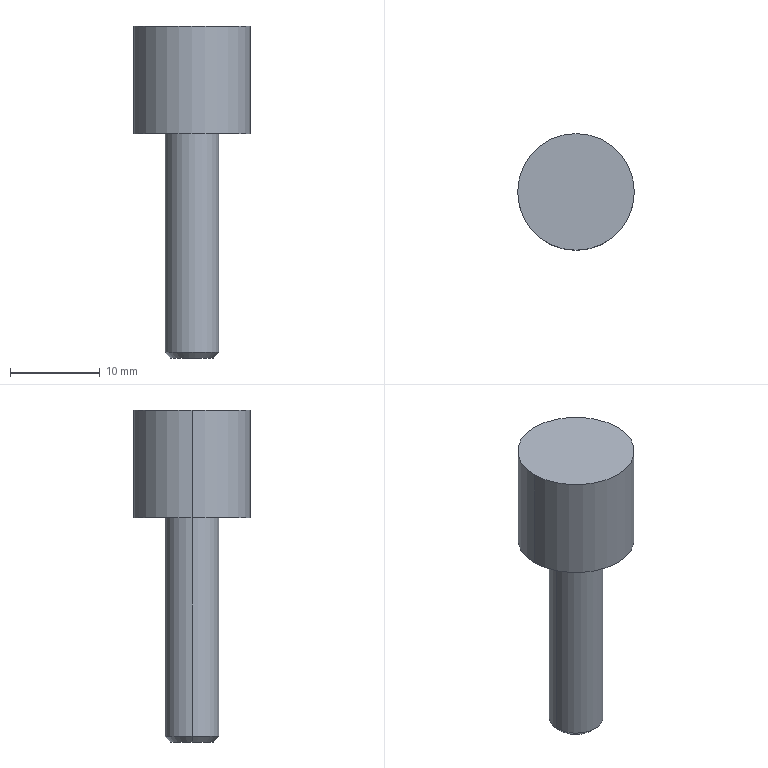Part | STEP file | LE-MX-A-TJG_PN_0007 | 1 solid | 9 faces | box 13 x 13 x 37 mm | volume 2296 mm3 | cylinder 4 | plane 3 | cone 2 | commonest cylinder face diameters 6 x2 13 x2
STEP:
#1=CARTESIAN_POINT('',(6.5,0.,0.));
#2=VERTEX_POINT('',#1);
#3=CARTESIAN_POINT('',(-6.5,0.,0.));
#4=VERTEX_POINT('',#3);
#5=CARTESIAN_POINT('',(0.,0.,0.));
#6=DIRECTION('',(0.,0.,1.));
#7=DIRECTION('',(1.,0.,0.));
#8=AXIS2_PLACEMENT_3D('',#5,#6,#7);
#9=CIRCLE('',#8,6.5);
#10=EDGE_CURVE('',#2,#4,#9,.T.);
#11=ORIENTED_EDGE('',*,*,#10,.T.);
#12=CARTESIAN_POINT('',(-6.5,0.,12.));
#13=VERTEX_POINT('',#12);
#14=CARTESIAN_POINT('',(-6.5,0.,-25.));
#15=DIRECTION('',(0.,0.,1.));
#16=VECTOR('',#15,1000.);
#17=LINE('',#14,#16);
#18=EDGE_CURVE('',#4,#13,#17,.T.);
#19=ORIENTED_EDGE('',*,*,#18,.T.);
#20=CARTESIAN_POINT('',(6.5,0.,12.));
#21=VERTEX_POINT('',#20);
#22=CARTESIAN_POINT('',(0.,0.,12.));
#23=DIRECTION('',(0.,0.,-1.));
#24=DIRECTION('',(1.,0.,0.));
#25=AXIS2_PLACEMENT_3D('',#22,#23,#24);
#26=CIRCLE('',#25,6.5);
#27=EDGE_CURVE('',#13,#21,#26,.T.);
#28=ORIENTED_EDGE('',*,*,#27,.T.);
#29=CARTESIAN_POINT('',(6.5,0.,-25.));
#30=DIRECTION('',(0.,0.,1.));
#31=VECTOR('',#30,1000.);
#32=LINE('',#29,#31);
#33=EDGE_CURVE('',#2,#21,#32,.T.);
#34=ORIENTED_EDGE('',*,*,#33,.F.);
#35=EDGE_LOOP('',(#11,#19,#28,#34));
#36=FACE_OUTER_BOUND('',#35,.T.);
#37=CARTESIAN_POINT('',(0.,0.,-25.));
#38=DIRECTION('',(0.,0.,1.));
#39=DIRECTION('',(1.,0.,0.));
#40=AXIS2_PLACEMENT_3D('',#37,#38,#39);
#41=CYLINDRICAL_SURFACE('',#40,6.5);
#42=ADVANCED_FACE('',(#36),#41,.T.);
#43=CARTESIAN_POINT('',(3.,0.,-24.387));
#44=VERTEX_POINT('',#43);
#45=CARTESIAN_POINT('',(-3.,0.,-24.387));
#46=VERTEX_POINT('',#45);
#47=CARTESIAN_POINT('',(0.,0.,-24.387));
#48=DIRECTION('',(0.,0.,1.));
#49=DIRECTION('',(1.,0.,0.));
#50=AXIS2_PLACEMENT_3D('',#47,#48,#49);
#51=CIRCLE('',#50,3.);
#52=EDGE_CURVE('',#44,#46,#51,.T.);
#53=ORIENTED_EDGE('',*,*,#52,.T.);
#54=CARTESIAN_POINT('',(-3.,0.,0.));
#55=VERTEX_POINT('',#54);
#56=CARTESIAN_POINT('',(-3.,0.,-25.));
#57=DIRECTION('',(0.,0.,1.));
#58=VECTOR('',#57,1000.);
#59=LINE('',#56,#58);
#60=EDGE_CURVE('',#46,#55,#59,.T.);
#61=ORIENTED_EDGE('',*,*,#60,.T.);
#62=CARTESIAN_POINT('',(3.,0.,0.));
#63=VERTEX_POINT('',#62);
#64=CARTESIAN_POINT('',(0.,0.,0.));
#65=DIRECTION('',(0.,0.,1.));
#66=DIRECTION('',(1.,0.,0.));
#67=AXIS2_PLACEMENT_3D('',#64,#65,#66);
#68=CIRCLE('',#67,3.);
#69=EDGE_CURVE('',#63,#55,#68,.T.);
#70=ORIENTED_EDGE('',*,*,#69,.F.);
#71=CARTESIAN_POINT('',(3.,0.,-25.));
#72=DIRECTION('',(0.,0.,1.));
#73=VECTOR('',#72,1000.);
#74=LINE('',#71,#73);
#75=EDGE_CURVE('',#44,#63,#74,.T.);
#76=ORIENTED_EDGE('',*,*,#75,.F.);
#77=EDGE_LOOP('',(#53,#61,#70,#76));
#78=FACE_OUTER_BOUND('',#77,.T.);
#79=CARTESIAN_POINT('',(0.,0.,-25.));
#80=DIRECTION('',(0.,0.,1.));
#81=DIRECTION('',(1.,0.,0.));
#82=AXIS2_PLACEMENT_3D('',#79,#80,#81);
#83=CYLINDRICAL_SURFACE('',#82,3.);
#84=ADVANCED_FACE('',(#78),#83,.T.);
#85=CARTESIAN_POINT('',(2.387,0.,-25.));
#86=VERTEX_POINT('',#85);
#87=CARTESIAN_POINT('',(-2.387,0.,-25.));
#88=VERTEX_POINT('',#87);
#89=CARTESIAN_POINT('',(0.,0.,-25.));
#90=DIRECTION('',(0.,0.,1.));
#91=DIRECTION('',(1.,0.,0.));
#92=AXIS2_PLACEMENT_3D('',#89,#90,#91);
#93=CIRCLE('',#92,2.387);
#94=EDGE_CURVE('',#86,#88,#93,.T.);
#95=ORIENTED_EDGE('',*,*,#94,.T.);
#96=CARTESIAN_POINT('',(-3.,0.,-24.387));
#97=DIRECTION('',(-0.7071,0.,0.7071));
#98=VECTOR('',#97,1000.);
#99=LINE('',#96,#98);
#100=EDGE_CURVE('',#88,#46,#99,.T.);
#101=ORIENTED_EDGE('',*,*,#100,.T.);
#102=ORIENTED_EDGE('',*,*,#52,.F.);
#103=CARTESIAN_POINT('',(3.,0.,-24.387));
#104=DIRECTION('',(0.7071,0.,0.7071));
#105=VECTOR('',#104,1000.);
#106=LINE('',#103,#105);
#107=EDGE_CURVE('',#86,#44,#106,.T.);
#108=ORIENTED_EDGE('',*,*,#107,.F.);
#109=EDGE_LOOP('',(#95,#101,#102,#108));
#110=FACE_OUTER_BOUND('',#109,.T.);
#111=CARTESIAN_POINT('',(0.,0.,-24.387));
#112=DIRECTION('',(0.,0.,1.));
#113=DIRECTION('',(1.,0.,0.));
#114=AXIS2_PLACEMENT_3D('',#111,#112,#113);
#115=CONICAL_SURFACE('',#114,3.,0.7854);
#116=ADVANCED_FACE('',(#110),#115,.T.);
#117=ORIENTED_EDGE('',*,*,#18,.F.);
#118=CARTESIAN_POINT('',(0.,0.,0.));
#119=DIRECTION('',(0.,0.,1.));
#120=DIRECTION('',(1.,0.,0.));
#121=AXIS2_PLACEMENT_3D('',#118,#119,#120);
#122=CIRCLE('',#121,6.5);
#123=EDGE_CURVE('',#4,#2,#122,.T.);
#124=ORIENTED_EDGE('',*,*,#123,.T.);
#125=ORIENTED_EDGE('',*,*,#33,.T.);
#126=CARTESIAN_POINT('',(0.,0.,12.));
#127=DIRECTION('',(0.,0.,-1.));
#128=DIRECTION('',(1.,0.,0.));
#129=AXIS2_PLACEMENT_3D('',#126,#127,#128);
#130=CIRCLE('',#129,6.5);
#131=EDGE_CURVE('',#21,#13,#130,.T.);
#132=ORIENTED_EDGE('',*,*,#131,.T.);
#133=EDGE_LOOP('',(#117,#124,#125,#132));
#134=FACE_OUTER_BOUND('',#133,.T.);
#135=CARTESIAN_POINT('',(0.,0.,-25.));
#136=DIRECTION('',(0.,0.,1.));
#137=DIRECTION('',(1.,0.,0.));
#138=AXIS2_PLACEMENT_3D('',#135,#136,#137);
#139=CYLINDRICAL_SURFACE('',#138,6.5);
#140=ADVANCED_FACE('',(#134),#139,.T.);
#141=ORIENTED_EDGE('',*,*,#131,.F.);
#142=ORIENTED_EDGE('',*,*,#27,.F.);
#143=EDGE_LOOP('',(#141,#142));
#144=FACE_OUTER_BOUND('',#143,.T.);
#145=CARTESIAN_POINT('',(0.,0.,12.));
#146=DIRECTION('',(0.,0.,1.));
#147=DIRECTION('',(1.,0.,0.));
#148=AXIS2_PLACEMENT_3D('',#145,#146,#147);
#149=PLANE('',#148);
#150=ADVANCED_FACE('',(#144),#149,.T.);
#151=ORIENTED_EDGE('',*,*,#10,.F.);
#152=ORIENTED_EDGE('',*,*,#123,.F.);
#153=EDGE_LOOP('',(#151,#152));
#154=FACE_OUTER_BOUND('',#153,.T.);
#155=ORIENTED_EDGE('',*,*,#69,.T.);
#156=CARTESIAN_POINT('',(0.,0.,0.));
#157=DIRECTION('',(0.,0.,1.));
#158=DIRECTION('',(1.,0.,0.));
#159=AXIS2_PLACEMENT_3D('',#156,#157,#158);
#160=CIRCLE('',#159,3.);
#161=EDGE_CURVE('',#55,#63,#160,.T.);
#162=ORIENTED_EDGE('',*,*,#161,.T.);
#163=EDGE_LOOP('',(#155,#162));
#164=FACE_BOUND('',#163,.T.);
#165=CARTESIAN_POINT('',(6.5,0.,0.));
#166=DIRECTION('',(0.,0.,-1.));
#167=DIRECTION('',(-1.,0.,0.));
#168=AXIS2_PLACEMENT_3D('',#165,#166,#167);
#169=PLANE('',#168);
#170=ADVANCED_FACE('',(#154,#164),#169,.T.);
#171=ORIENTED_EDGE('',*,*,#60,.F.);
#172=CARTESIAN_POINT('',(0.,0.,-24.387));
#173=DIRECTION('',(0.,0.,1.));
#174=DIRECTION('',(1.,0.,0.));
#175=AXIS2_PLACEMENT_3D('',#172,#173,#174);
#176=CIRCLE('',#175,3.);
#177=EDGE_CURVE('',#46,#44,#176,.T.);
#178=ORIENTED_EDGE('',*,*,#177,.T.);
#179=ORIENTED_EDGE('',*,*,#75,.T.);
#180=ORIENTED_EDGE('',*,*,#161,.F.);
#181=EDGE_LOOP('',(#171,#178,#179,#180));
#182=FACE_OUTER_BOUND('',#181,.T.);
#183=CARTESIAN_POINT('',(0.,0.,-25.));
#184=DIRECTION('',(0.,0.,1.));
#185=DIRECTION('',(1.,0.,0.));
#186=AXIS2_PLACEMENT_3D('',#183,#184,#185);
#187=CYLINDRICAL_SURFACE('',#186,3.);
#188=ADVANCED_FACE('',(#182),#187,.T.);
#189=ORIENTED_EDGE('',*,*,#100,.F.);
#190=CARTESIAN_POINT('',(0.,0.,-25.));
#191=DIRECTION('',(0.,0.,1.));
#192=DIRECTION('',(1.,0.,0.));
#193=AXIS2_PLACEMENT_3D('',#190,#191,#192);
#194=CIRCLE('',#193,2.387);
#195=EDGE_CURVE('',#88,#86,#194,.T.);
#196=ORIENTED_EDGE('',*,*,#195,.T.);
#197=ORIENTED_EDGE('',*,*,#107,.T.);
#198=ORIENTED_EDGE('',*,*,#177,.F.);
#199=EDGE_LOOP('',(#189,#196,#197,#198));
#200=FACE_OUTER_BOUND('',#199,.T.);
#201=CARTESIAN_POINT('',(0.,0.,-24.387));
#202=DIRECTION('',(0.,0.,1.));
#203=DIRECTION('',(1.,0.,0.));
#204=AXIS2_PLACEMENT_3D('',#201,#202,#203);
#205=CONICAL_SURFACE('',#204,3.,0.7854);
#206=ADVANCED_FACE('',(#200),#205,.T.);
#207=ORIENTED_EDGE('',*,*,#94,.F.);
#208=ORIENTED_EDGE('',*,*,#195,.F.);
#209=EDGE_LOOP('',(#207,#208));
#210=FACE_OUTER_BOUND('',#209,.T.);
#211=CARTESIAN_POINT('',(2.387,0.,-25.));
#212=DIRECTION('',(0.,0.,-1.));
#213=DIRECTION('',(-1.,0.,0.));
#214=AXIS2_PLACEMENT_3D('',#211,#212,#213);
#215=PLANE('',#214);
#216=ADVANCED_FACE('',(#210),#215,.T.);
#217=CLOSED_SHELL('',(#42,#84,#116,#140,#150,#170,#188,#206,#216));
#218=MANIFOLD_SOLID_BREP('',#217);
#219=CARTESIAN_POINT('',(0.,0.,0.));
#220=DIRECTION('',(0.,0.,1.));
#221=DIRECTION('',(1.,0.,0.));
#222=AXIS2_PLACEMENT_3D('',#219,#220,#221);
#223=(LENGTH_UNIT()NAMED_UNIT(*)SI_UNIT(.MILLI.,.METRE.));
#224=UNCERTAINTY_MEASURE_WITH_UNIT(LENGTH_MEASURE(0.00001),#223,'','');
#225=(NAMED_UNIT(*)PLANE_ANGLE_UNIT()SI_UNIT($,.RADIAN.));
#226=(NAMED_UNIT(*)SI_UNIT($,.STERADIAN.)SOLID_ANGLE_UNIT());
#227=(GEOMETRIC_REPRESENTATION_CONTEXT(3)GLOBAL_UNCERTAINTY_ASSIGNED_CONTEXT((#224))GLOBAL_UNIT_ASSIGNED_CONTEXT((#223,#225,#226))REPRESENTATION_CONTEXT('',''));
#228=ADVANCED_BREP_SHAPE_REPRESENTATION('',(#218,#222),#227);